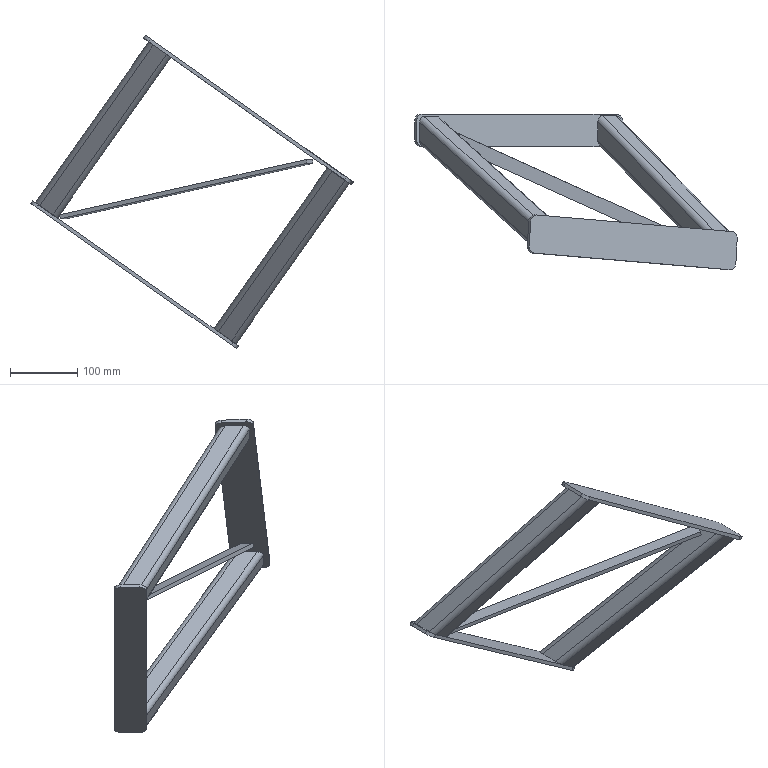Part | STEP file | upper-lower conveyor link bracket right | 5 solids | 62 faces | box 481.108 x 232.016 x 467.858 mm | volume 606550 mm3 | plane 38 | cylinder 24 | commonest cylinder face diameters 8 x8 16 x8 20 x8